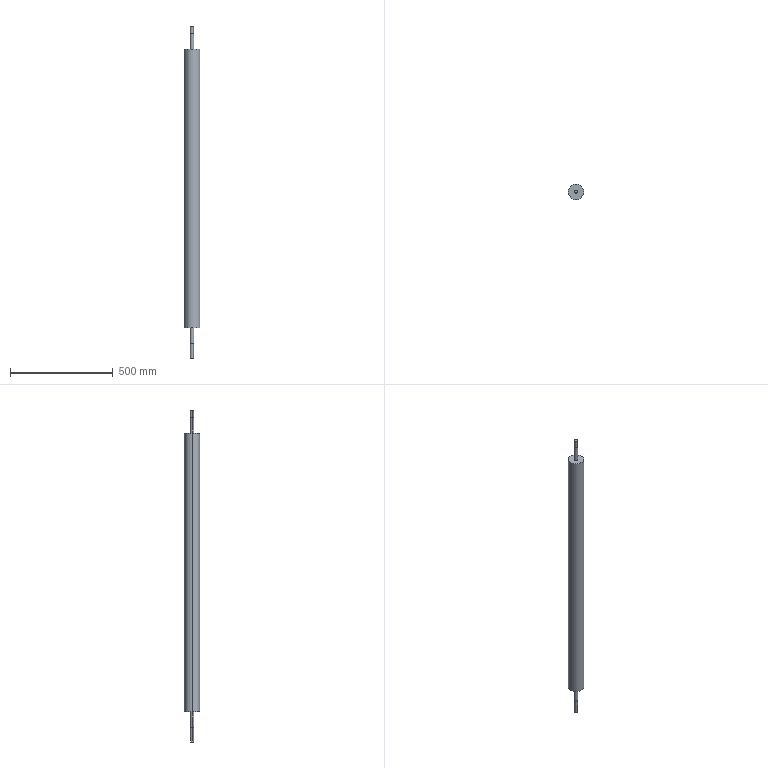Part | SolidWorks | features ICE 5, MirrorPattern 2, Extrusion 1 | 1 solid | 21 faces | box 76 x 76 x 1615 mm | volume 6202615 mm3 | cylinder 12 | plane 9 | commonest cylinder face diameters 15 x4 16.5 x4 5 x2 76 x2
STEP:
#1=CARTESIAN_POINT('',(2.5,4.5,-809.75));
#2=VERTEX_POINT('',#1);
#3=CARTESIAN_POINT('',(0.,4.5,-807.25));
#4=VERTEX_POINT('',#3);
#5=CARTESIAN_POINT('',(0.,4.5,-809.75));
#6=DIRECTION('',(0.,-1.,0.));
#7=DIRECTION('',(0.,0.,-1.));
#8=AXIS2_PLACEMENT_3D('',#5,#6,#7);
#9=CIRCLE('',#8,2.5);
#10=EDGE_CURVE('',#2,#4,#9,.T.);
#11=ORIENTED_EDGE('',*,*,#10,.T.);
#12=CARTESIAN_POINT('',(0.,7.5,-807.25));
#13=VERTEX_POINT('',#12);
#14=CARTESIAN_POINT('',(0.,4.5,-807.25));
#15=DIRECTION('',(0.,1.,0.));
#16=VECTOR('',#15,1000.);
#17=LINE('',#14,#16);
#18=EDGE_CURVE('',#4,#13,#17,.T.);
#19=ORIENTED_EDGE('',*,*,#18,.T.);
#20=CARTESIAN_POINT('',(2.5,7.071,-809.75));
#21=VERTEX_POINT('',#20);
#22=CARTESIAN_POINT('',(2.5,7.071,-809.75));
#23=CARTESIAN_POINT('',(2.5,7.071,-809.583));
#24=CARTESIAN_POINT('',(2.484,7.077,-809.42));
#25=CARTESIAN_POINT('',(2.419,7.099,-809.099));
#26=CARTESIAN_POINT('',(2.371,7.116,-808.939));
#27=CARTESIAN_POINT('',(2.245,7.157,-808.637));
#28=CARTESIAN_POINT('',(2.168,7.181,-808.494));
#29=CARTESIAN_POINT('',(1.986,7.233,-808.223));
#30=CARTESIAN_POINT('',(1.882,7.261,-808.096));
#31=CARTESIAN_POINT('',(1.538,7.344,-807.753));
#32=CARTESIAN_POINT('',(1.261,7.399,-807.567));
#33=CARTESIAN_POINT('',(0.81,7.458,-807.379));
#34=CARTESIAN_POINT('',(0.6511,7.473,-807.331));
#35=CARTESIAN_POINT('',(0.3276,7.495,-807.266));
#36=CARTESIAN_POINT('',(0.1645,7.5,-807.25));
#37=CARTESIAN_POINT('',(0.,7.5,-807.25));
#38=B_SPLINE_CURVE_WITH_KNOTS('',3,(#22,#23,#24,#25,#26,#27,#28,#29,#30,#31,#32,#33,#34,#35,#36,#37),.UNSPECIFIED.,.F.,.F.,(4,2,2,2,2,2,2,4),(0.,0.0004922,0.0009844,0.001477,0.001969,0.002953,0.003445,0.003937),.UNSPECIFIED.);
#39=EDGE_CURVE('',#21,#13,#38,.T.);
#40=ORIENTED_EDGE('',*,*,#39,.F.);
#41=CARTESIAN_POINT('',(2.5,4.5,-809.75));
#42=DIRECTION('',(0.,1.,0.));
#43=VECTOR('',#42,1000.);
#44=LINE('',#41,#43);
#45=EDGE_CURVE('',#2,#21,#44,.T.);
#46=ORIENTED_EDGE('',*,*,#45,.F.);
#47=EDGE_LOOP('',(#11,#19,#40,#46));
#48=FACE_OUTER_BOUND('',#47,.T.);
#49=CARTESIAN_POINT('',(0.,4.5,-809.75));
#50=DIRECTION('',(0.,1.,0.));
#51=DIRECTION('',(0.,0.,1.));
#52=AXIS2_PLACEMENT_3D('',#49,#50,#51);
#53=CYLINDRICAL_SURFACE('',#52,2.5);
#54=ADVANCED_FACE('',(#48),#53,.F.);
#55=CARTESIAN_POINT('',(-8.25,0.,-754.));
#56=VERTEX_POINT('',#55);
#57=CARTESIAN_POINT('',(8.25,0.,-754.));
#58=VERTEX_POINT('',#57);
#59=CARTESIAN_POINT('',(0.,0.,-754.));
#60=DIRECTION('',(0.,0.,-1.));
#61=DIRECTION('',(-1.,0.,0.));
#62=AXIS2_PLACEMENT_3D('',#59,#60,#61);
#63=CIRCLE('',#62,8.25);
#64=EDGE_CURVE('',#56,#58,#63,.T.);
#65=ORIENTED_EDGE('',*,*,#64,.F.);
#66=CARTESIAN_POINT('',(-8.25,0.,-678.));
#67=VERTEX_POINT('',#66);
#68=CARTESIAN_POINT('',(-8.25,0.,-754.));
#69=DIRECTION('',(0.,0.,1.));
#70=VECTOR('',#69,1000.);
#71=LINE('',#68,#70);
#72=EDGE_CURVE('',#56,#67,#71,.T.);
#73=ORIENTED_EDGE('',*,*,#72,.T.);
#74=CARTESIAN_POINT('',(8.25,0.,-678.));
#75=VERTEX_POINT('',#74);
#76=CARTESIAN_POINT('',(0.,0.,-678.));
#77=DIRECTION('',(0.,0.,-1.));
#78=DIRECTION('',(1.,0.,0.));
#79=AXIS2_PLACEMENT_3D('',#76,#77,#78);
#80=CIRCLE('',#79,8.25);
#81=EDGE_CURVE('',#67,#75,#80,.T.);
#82=ORIENTED_EDGE('',*,*,#81,.T.);
#83=CARTESIAN_POINT('',(8.25,0.,-754.));
#84=DIRECTION('',(0.,0.,1.));
#85=VECTOR('',#84,1000.);
#86=LINE('',#83,#85);
#87=EDGE_CURVE('',#58,#75,#86,.T.);
#88=ORIENTED_EDGE('',*,*,#87,.F.);
#89=EDGE_LOOP('',(#65,#73,#82,#88));
#90=FACE_OUTER_BOUND('',#89,.T.);
#91=CARTESIAN_POINT('',(0.,0.,-754.));
#92=DIRECTION('',(0.,0.,1.));
#93=DIRECTION('',(1.,0.,0.));
#94=AXIS2_PLACEMENT_3D('',#91,#92,#93);
#95=CYLINDRICAL_SURFACE('',#94,8.25);
#96=ADVANCED_FACE('',(#90),#95,.T.);
#97=CARTESIAN_POINT('',(8.25,0.,754.));
#98=VERTEX_POINT('',#97);
#99=CARTESIAN_POINT('',(-8.25,0.,754.));
#100=VERTEX_POINT('',#99);
#101=CARTESIAN_POINT('',(0.,0.,754.));
#102=DIRECTION('',(0.,0.,1.));
#103=DIRECTION('',(1.,0.,0.));
#104=AXIS2_PLACEMENT_3D('',#101,#102,#103);
#105=CIRCLE('',#104,8.25);
#106=EDGE_CURVE('',#98,#100,#105,.T.);
#107=ORIENTED_EDGE('',*,*,#106,.F.);
#108=CARTESIAN_POINT('',(8.25,0.,678.));
#109=VERTEX_POINT('',#108);
#110=CARTESIAN_POINT('',(8.25,0.,754.));
#111=DIRECTION('',(0.,0.,-1.));
#112=VECTOR('',#111,1000.);
#113=LINE('',#110,#112);
#114=EDGE_CURVE('',#98,#109,#113,.T.);
#115=ORIENTED_EDGE('',*,*,#114,.T.);
#116=CARTESIAN_POINT('',(-8.25,0.,678.));
#117=VERTEX_POINT('',#116);
#118=CARTESIAN_POINT('',(0.,0.,678.));
#119=DIRECTION('',(0.,0.,1.));
#120=DIRECTION('',(1.,0.,0.));
#121=AXIS2_PLACEMENT_3D('',#118,#119,#120);
#122=CIRCLE('',#121,8.25);
#123=EDGE_CURVE('',#109,#117,#122,.T.);
#124=ORIENTED_EDGE('',*,*,#123,.T.);
#125=CARTESIAN_POINT('',(-8.25,0.,754.));
#126=DIRECTION('',(0.,0.,-1.));
#127=VECTOR('',#126,1000.);
#128=LINE('',#125,#127);
#129=EDGE_CURVE('',#100,#117,#128,.T.);
#130=ORIENTED_EDGE('',*,*,#129,.F.);
#131=EDGE_LOOP('',(#107,#115,#124,#130));
#132=FACE_OUTER_BOUND('',#131,.T.);
#133=CARTESIAN_POINT('',(0.,0.,754.));
#134=DIRECTION('',(0.,0.,-1.));
#135=DIRECTION('',(-1.,0.,0.));
#136=AXIS2_PLACEMENT_3D('',#133,#134,#135);
#137=CYLINDRICAL_SURFACE('',#136,8.25);
#138=ADVANCED_FACE('',(#132),#137,.T.);
#139=CARTESIAN_POINT('',(38.,0.,678.));
#140=VERTEX_POINT('',#139);
#141=CARTESIAN_POINT('',(-38.,0.,678.));
#142=VERTEX_POINT('',#141);
#143=CARTESIAN_POINT('',(0.,0.,678.));
#144=DIRECTION('',(0.,0.,1.));
#145=DIRECTION('',(1.,0.,0.));
#146=AXIS2_PLACEMENT_3D('',#143,#144,#145);
#147=CIRCLE('',#146,38.);
#148=EDGE_CURVE('',#140,#142,#147,.T.);
#149=ORIENTED_EDGE('',*,*,#148,.F.);
#150=CARTESIAN_POINT('',(38.,0.,-678.));
#151=VERTEX_POINT('',#150);
#152=CARTESIAN_POINT('',(38.,0.,678.));
#153=DIRECTION('',(0.,0.,-1.));
#154=VECTOR('',#153,1000.);
#155=LINE('',#152,#154);
#156=EDGE_CURVE('',#140,#151,#155,.T.);
#157=ORIENTED_EDGE('',*,*,#156,.T.);
#158=CARTESIAN_POINT('',(-38.,0.,-678.));
#159=VERTEX_POINT('',#158);
#160=CARTESIAN_POINT('',(0.,0.,-678.));
#161=DIRECTION('',(0.,0.,1.));
#162=DIRECTION('',(1.,0.,0.));
#163=AXIS2_PLACEMENT_3D('',#160,#161,#162);
#164=CIRCLE('',#163,38.);
#165=EDGE_CURVE('',#151,#159,#164,.T.);
#166=ORIENTED_EDGE('',*,*,#165,.T.);
#167=CARTESIAN_POINT('',(-38.,0.,678.));
#168=DIRECTION('',(0.,0.,-1.));
#169=VECTOR('',#168,1000.);
#170=LINE('',#167,#169);
#171=EDGE_CURVE('',#142,#159,#170,.T.);
#172=ORIENTED_EDGE('',*,*,#171,.F.);
#173=EDGE_LOOP('',(#149,#157,#166,#172));
#174=FACE_OUTER_BOUND('',#173,.T.);
#175=CARTESIAN_POINT('',(0.,0.,678.));
#176=DIRECTION('',(0.,0.,-1.));
#177=DIRECTION('',(-1.,0.,0.));
#178=AXIS2_PLACEMENT_3D('',#175,#176,#177);
#179=CYLINDRICAL_SURFACE('',#178,38.);
#180=ADVANCED_FACE('',(#174),#179,.T.);
#181=CARTESIAN_POINT('',(-2.5,7.071,-824.75));
#182=VERTEX_POINT('',#181);
#183=CARTESIAN_POINT('',(-7.5,0.,-824.75));
#184=VERTEX_POINT('',#183);
#185=CARTESIAN_POINT('',(0.,0.,-824.75));
#186=DIRECTION('',(0.,0.,1.));
#187=DIRECTION('',(1.,0.,0.));
#188=AXIS2_PLACEMENT_3D('',#185,#186,#187);
#189=CIRCLE('',#188,7.5);
#190=EDGE_CURVE('',#182,#184,#189,.T.);
#191=ORIENTED_EDGE('',*,*,#190,.T.);
#192=CARTESIAN_POINT('',(-7.5,0.,-754.));
#193=VERTEX_POINT('',#192);
#194=CARTESIAN_POINT('',(-7.5,0.,-824.75));
#195=DIRECTION('',(0.,0.,1.));
#196=VECTOR('',#195,1000.);
#197=LINE('',#194,#196);
#198=EDGE_CURVE('',#184,#193,#197,.T.);
#199=ORIENTED_EDGE('',*,*,#198,.T.);
#200=CARTESIAN_POINT('',(7.5,0.,-754.));
#201=VERTEX_POINT('',#200);
#202=CARTESIAN_POINT('',(0.,0.,-754.));
#203=DIRECTION('',(0.,0.,1.));
#204=DIRECTION('',(-1.,0.,0.));
#205=AXIS2_PLACEMENT_3D('',#202,#203,#204);
#206=CIRCLE('',#205,7.5);
#207=EDGE_CURVE('',#201,#193,#206,.T.);
#208=ORIENTED_EDGE('',*,*,#207,.F.);
#209=CARTESIAN_POINT('',(7.5,0.,-824.75));
#210=VERTEX_POINT('',#209);
#211=CARTESIAN_POINT('',(7.5,0.,-824.75));
#212=DIRECTION('',(0.,0.,1.));
#213=VECTOR('',#212,1000.);
#214=LINE('',#211,#213);
#215=EDGE_CURVE('',#210,#201,#214,.T.);
#216=ORIENTED_EDGE('',*,*,#215,.F.);
#217=CARTESIAN_POINT('',(2.5,7.071,-824.75));
#218=VERTEX_POINT('',#217);
#219=CARTESIAN_POINT('',(0.,0.,-824.75));
#220=DIRECTION('',(0.,0.,1.));
#221=DIRECTION('',(1.,0.,0.));
#222=AXIS2_PLACEMENT_3D('',#219,#220,#221);
#223=CIRCLE('',#222,7.5);
#224=EDGE_CURVE('',#210,#218,#223,.T.);
#225=ORIENTED_EDGE('',*,*,#224,.T.);
#226=CARTESIAN_POINT('',(2.5,7.071,-824.75));
#227=DIRECTION('',(0.,0.,1.));
#228=VECTOR('',#227,1000.);
#229=LINE('',#226,#228);
#230=EDGE_CURVE('',#218,#21,#229,.T.);
#231=ORIENTED_EDGE('',*,*,#230,.T.);
#232=ORIENTED_EDGE('',*,*,#39,.T.);
#233=CARTESIAN_POINT('',(-2.5,7.071,-809.75));
#234=VERTEX_POINT('',#233);
#235=CARTESIAN_POINT('',(0.,7.5,-807.25));
#236=CARTESIAN_POINT('',(-0.1643,7.5,-807.25));
#237=CARTESIAN_POINT('',(-0.3311,7.494,-807.267));
#238=CARTESIAN_POINT('',(-0.6524,7.473,-807.331));
#239=CARTESIAN_POINT('',(-0.8088,7.458,-807.379));
#240=CARTESIAN_POINT('',(-1.113,7.419,-807.505));
#241=CARTESIAN_POINT('',(-1.257,7.395,-807.583));
#242=CARTESIAN_POINT('',(-1.526,7.344,-807.763));
#243=CARTESIAN_POINT('',(-1.653,7.316,-807.868));
#244=CARTESIAN_POINT('',(-1.883,7.261,-808.098));
#245=CARTESIAN_POINT('',(-1.986,7.233,-808.223));
#246=CARTESIAN_POINT('',(-2.167,7.181,-808.492));
#247=CARTESIAN_POINT('',(-2.245,7.156,-808.638));
#248=CARTESIAN_POINT('',(-2.37,7.116,-808.939));
#249=CARTESIAN_POINT('',(-2.418,7.1,-809.094));
#250=CARTESIAN_POINT('',(-2.483,7.077,-809.418));
#251=CARTESIAN_POINT('',(-2.5,7.071,-809.584));
#252=CARTESIAN_POINT('',(-2.5,7.071,-809.75));
#253=B_SPLINE_CURVE_WITH_KNOTS('',3,(#235,#236,#237,#238,#239,#240,#241,#242,#243,#244,#245,#246,#247,#248,#249,#250,#251,#252),.UNSPECIFIED.,.F.,.F.,(4,2,2,2,2,2,2,2,4),(0.003937,0.004429,0.004921,0.005412,0.005904,0.006395,0.006887,0.007378,0.00787),.UNSPECIFIED.);
#254=EDGE_CURVE('',#13,#234,#253,.T.);
#255=ORIENTED_EDGE('',*,*,#254,.T.);
#256=CARTESIAN_POINT('',(-2.5,7.071,-824.75));
#257=DIRECTION('',(0.,0.,-1.));
#258=VECTOR('',#257,1000.);
#259=LINE('',#256,#258);
#260=EDGE_CURVE('',#234,#182,#259,.T.);
#261=ORIENTED_EDGE('',*,*,#260,.T.);
#262=EDGE_LOOP('',(#191,#199,#208,#216,#225,#231,#232,#255,#261));
#263=FACE_OUTER_BOUND('',#262,.T.);
#264=CARTESIAN_POINT('',(0.,0.,-824.75));
#265=DIRECTION('',(0.,0.,1.));
#266=DIRECTION('',(1.,0.,0.));
#267=AXIS2_PLACEMENT_3D('',#264,#265,#266);
#268=CYLINDRICAL_SURFACE('',#267,7.5);
#269=ADVANCED_FACE('',(#263),#268,.T.);
#270=CARTESIAN_POINT('',(7.5,0.,790.3));
#271=VERTEX_POINT('',#270);
#272=CARTESIAN_POINT('',(-7.5,0.,790.3));
#273=VERTEX_POINT('',#272);
#274=CARTESIAN_POINT('',(0.,0.,790.3));
#275=DIRECTION('',(0.,0.,1.));
#276=DIRECTION('',(1.,0.,0.));
#277=AXIS2_PLACEMENT_3D('',#274,#275,#276);
#278=CIRCLE('',#277,7.5);
#279=EDGE_CURVE('',#271,#273,#278,.T.);
#280=ORIENTED_EDGE('',*,*,#279,.F.);
#281=CARTESIAN_POINT('',(7.5,0.,754.));
#282=VERTEX_POINT('',#281);
#283=CARTESIAN_POINT('',(7.5,0.,824.75));
#284=DIRECTION('',(0.,0.,-1.));
#285=VECTOR('',#284,1000.);
#286=LINE('',#283,#285);
#287=EDGE_CURVE('',#271,#282,#286,.T.);
#288=ORIENTED_EDGE('',*,*,#287,.T.);
#289=CARTESIAN_POINT('',(-7.5,0.,754.));
#290=VERTEX_POINT('',#289);
#291=CARTESIAN_POINT('',(0.,0.,754.));
#292=DIRECTION('',(0.,0.,1.));
#293=DIRECTION('',(1.,0.,0.));
#294=AXIS2_PLACEMENT_3D('',#291,#292,#293);
#295=CIRCLE('',#294,7.5);
#296=EDGE_CURVE('',#282,#290,#295,.T.);
#297=ORIENTED_EDGE('',*,*,#296,.T.);
#298=CARTESIAN_POINT('',(-7.5,0.,824.75));
#299=DIRECTION('',(0.,0.,-1.));
#300=VECTOR('',#299,1000.);
#301=LINE('',#298,#300);
#302=EDGE_CURVE('',#273,#290,#301,.T.);
#303=ORIENTED_EDGE('',*,*,#302,.F.);
#304=EDGE_LOOP('',(#280,#288,#297,#303));
#305=FACE_OUTER_BOUND('',#304,.T.);
#306=CARTESIAN_POINT('',(0.,0.,824.75));
#307=DIRECTION('',(0.,0.,-1.));
#308=DIRECTION('',(-1.,0.,0.));
#309=AXIS2_PLACEMENT_3D('',#306,#307,#308);
#310=CYLINDRICAL_SURFACE('',#309,7.5);
#311=ADVANCED_FACE('',(#305),#310,.T.);
#312=ORIENTED_EDGE('',*,*,#287,.F.);
#313=CARTESIAN_POINT('',(0.,0.,790.3));
#314=DIRECTION('',(0.,0.,1.));
#315=DIRECTION('',(1.,0.,0.));
#316=AXIS2_PLACEMENT_3D('',#313,#314,#315);
#317=CIRCLE('',#316,7.5);
#318=EDGE_CURVE('',#273,#271,#317,.T.);
#319=ORIENTED_EDGE('',*,*,#318,.F.);
#320=ORIENTED_EDGE('',*,*,#302,.T.);
#321=CARTESIAN_POINT('',(0.,0.,754.));
#322=DIRECTION('',(0.,0.,1.));
#323=DIRECTION('',(1.,0.,0.));
#324=AXIS2_PLACEMENT_3D('',#321,#322,#323);
#325=CIRCLE('',#324,7.5);
#326=EDGE_CURVE('',#290,#282,#325,.T.);
#327=ORIENTED_EDGE('',*,*,#326,.T.);
#328=EDGE_LOOP('',(#312,#319,#320,#327));
#329=FACE_OUTER_BOUND('',#328,.T.);
#330=CARTESIAN_POINT('',(0.,0.,824.75));
#331=DIRECTION('',(0.,0.,-1.));
#332=DIRECTION('',(-1.,0.,0.));
#333=AXIS2_PLACEMENT_3D('',#330,#331,#332);
#334=CYLINDRICAL_SURFACE('',#333,7.5);
#335=ADVANCED_FACE('',(#329),#334,.T.);
#336=CARTESIAN_POINT('',(-2.5,4.5,-824.75));
#337=VERTEX_POINT('',#336);
#338=CARTESIAN_POINT('',(2.5,4.5,-824.75));
#339=VERTEX_POINT('',#338);
#340=CARTESIAN_POINT('',(0.,4.5,-824.75));
#341=DIRECTION('',(1.,0.,0.));
#342=VECTOR('',#341,1000.);
#343=LINE('',#340,#342);
#344=EDGE_CURVE('',#337,#339,#343,.T.);
#345=ORIENTED_EDGE('',*,*,#344,.T.);
#346=CARTESIAN_POINT('',(2.5,4.5,-824.75));
#347=DIRECTION('',(0.,1.,0.));
#348=VECTOR('',#347,1000.);
#349=LINE('',#346,#348);
#350=EDGE_CURVE('',#339,#218,#349,.T.);
#351=ORIENTED_EDGE('',*,*,#350,.T.);
#352=ORIENTED_EDGE('',*,*,#224,.F.);
#353=CARTESIAN_POINT('',(0.,0.,-824.75));
#354=DIRECTION('',(0.,0.,1.));
#355=DIRECTION('',(1.,0.,0.));
#356=AXIS2_PLACEMENT_3D('',#353,#354,#355);
#357=CIRCLE('',#356,7.5);
#358=EDGE_CURVE('',#184,#210,#357,.T.);
#359=ORIENTED_EDGE('',*,*,#358,.F.);
#360=ORIENTED_EDGE('',*,*,#190,.F.);
#361=CARTESIAN_POINT('',(-2.5,4.5,-824.75));
#362=DIRECTION('',(0.,1.,0.));
#363=VECTOR('',#362,1000.);
#364=LINE('',#361,#363);
#365=EDGE_CURVE('',#337,#182,#364,.T.);
#366=ORIENTED_EDGE('',*,*,#365,.F.);
#367=EDGE_LOOP('',(#345,#351,#352,#359,#360,#366));
#368=FACE_OUTER_BOUND('',#367,.T.);
#369=CARTESIAN_POINT('',(0.,0.,-824.75));
#370=DIRECTION('',(0.,0.,-1.));
#371=DIRECTION('',(1.,0.,0.));
#372=AXIS2_PLACEMENT_3D('',#369,#370,#371);
#373=PLANE('',#372);
#374=ADVANCED_FACE('',(#368),#373,.T.);
#375=ORIENTED_EDGE('',*,*,#198,.F.);
#376=ORIENTED_EDGE('',*,*,#358,.T.);
#377=ORIENTED_EDGE('',*,*,#215,.T.);
#378=CARTESIAN_POINT('',(0.,0.,-754.));
#379=DIRECTION('',(0.,0.,1.));
#380=DIRECTION('',(-1.,0.,0.));
#381=AXIS2_PLACEMENT_3D('',#378,#379,#380);
#382=CIRCLE('',#381,7.5);
#383=EDGE_CURVE('',#193,#201,#382,.T.);
#384=ORIENTED_EDGE('',*,*,#383,.F.);
#385=EDGE_LOOP('',(#375,#376,#377,#384));
#386=FACE_OUTER_BOUND('',#385,.T.);
#387=CARTESIAN_POINT('',(0.,0.,-824.75));
#388=DIRECTION('',(0.,0.,1.));
#389=DIRECTION('',(1.,0.,0.));
#390=AXIS2_PLACEMENT_3D('',#387,#388,#389);
#391=CYLINDRICAL_SURFACE('',#390,7.5);
#392=ADVANCED_FACE('',(#386),#391,.T.);
#393=ORIENTED_EDGE('',*,*,#156,.F.);
#394=CARTESIAN_POINT('',(0.,0.,678.));
#395=DIRECTION('',(0.,0.,1.));
#396=DIRECTION('',(1.,0.,0.));
#397=AXIS2_PLACEMENT_3D('',#394,#395,#396);
#398=CIRCLE('',#397,38.);
#399=EDGE_CURVE('',#142,#140,#398,.T.);
#400=ORIENTED_EDGE('',*,*,#399,.F.);
#401=ORIENTED_EDGE('',*,*,#171,.T.);
#402=CARTESIAN_POINT('',(0.,0.,-678.));
#403=DIRECTION('',(0.,0.,1.));
#404=DIRECTION('',(1.,0.,0.));
#405=AXIS2_PLACEMENT_3D('',#402,#403,#404);
#406=CIRCLE('',#405,38.);
#407=EDGE_CURVE('',#159,#151,#406,.T.);
#408=ORIENTED_EDGE('',*,*,#407,.T.);
#409=EDGE_LOOP('',(#393,#400,#401,#408));
#410=FACE_OUTER_BOUND('',#409,.T.);
#411=CARTESIAN_POINT('',(0.,0.,678.));
#412=DIRECTION('',(0.,0.,-1.));
#413=DIRECTION('',(-1.,0.,0.));
#414=AXIS2_PLACEMENT_3D('',#411,#412,#413);
#415=CYLINDRICAL_SURFACE('',#414,38.);
#416=ADVANCED_FACE('',(#410),#415,.T.);
#417=CARTESIAN_POINT('',(0.,0.,678.));
#418=DIRECTION('',(0.,0.,1.));
#419=DIRECTION('',(1.,0.,0.));
#420=AXIS2_PLACEMENT_3D('',#417,#418,#419);
#421=CIRCLE('',#420,8.25);
#422=EDGE_CURVE('',#117,#109,#421,.T.);
#423=ORIENTED_EDGE('',*,*,#422,.F.);
#424=ORIENTED_EDGE('',*,*,#123,.F.);
#425=EDGE_LOOP('',(#423,#424));
#426=FACE_BOUND('',#425,.T.);
#427=ORIENTED_EDGE('',*,*,#399,.T.);
#428=ORIENTED_EDGE('',*,*,#148,.T.);
#429=EDGE_LOOP('',(#427,#428));
#430=FACE_OUTER_BOUND('',#429,.T.);
#431=CARTESIAN_POINT('',(0.,0.,678.));
#432=DIRECTION('',(0.,0.,1.));
#433=DIRECTION('',(1.,0.,0.));
#434=AXIS2_PLACEMENT_3D('',#431,#432,#433);
#435=PLANE('',#434);
#436=ADVANCED_FACE('',(#426,#430),#435,.T.);
#437=CARTESIAN_POINT('',(0.,0.,-678.));
#438=DIRECTION('',(0.,0.,-1.));
#439=DIRECTION('',(1.,0.,0.));
#440=AXIS2_PLACEMENT_3D('',#437,#438,#439);
#441=CIRCLE('',#440,8.25);
#442=EDGE_CURVE('',#75,#67,#441,.T.);
#443=ORIENTED_EDGE('',*,*,#442,.F.);
#444=ORIENTED_EDGE('',*,*,#81,.F.);
#445=EDGE_LOOP('',(#443,#444));
#446=FACE_BOUND('',#445,.T.);
#447=ORIENTED_EDGE('',*,*,#407,.F.);
#448=ORIENTED_EDGE('',*,*,#165,.F.);
#449=EDGE_LOOP('',(#447,#448));
#450=FACE_OUTER_BOUND('',#449,.T.);
#451=CARTESIAN_POINT('',(0.,0.,-678.));
#452=DIRECTION('',(0.,0.,1.));
#453=DIRECTION('',(1.,0.,0.));
#454=AXIS2_PLACEMENT_3D('',#451,#452,#453);
#455=PLANE('',#454);
#456=ADVANCED_FACE('',(#446,#450),#455,.F.);
#457=ORIENTED_EDGE('',*,*,#114,.F.);
#458=CARTESIAN_POINT('',(0.,0.,754.));
#459=DIRECTION('',(0.,0.,1.));
#460=DIRECTION('',(1.,0.,0.));
#461=AXIS2_PLACEMENT_3D('',#458,#459,#460);
#462=CIRCLE('',#461,8.25);
#463=EDGE_CURVE('',#100,#98,#462,.T.);
#464=ORIENTED_EDGE('',*,*,#463,.F.);
#465=ORIENTED_EDGE('',*,*,#129,.T.);
#466=ORIENTED_EDGE('',*,*,#422,.T.);
#467=EDGE_LOOP('',(#457,#464,#465,#466));
#468=FACE_OUTER_BOUND('',#467,.T.);
#469=CARTESIAN_POINT('',(0.,0.,754.));
#470=DIRECTION('',(0.,0.,-1.));
#471=DIRECTION('',(-1.,0.,0.));
#472=AXIS2_PLACEMENT_3D('',#469,#470,#471);
#473=CYLINDRICAL_SURFACE('',#472,8.25);
#474=ADVANCED_FACE('',(#468),#473,.T.);
#475=ORIENTED_EDGE('',*,*,#326,.F.);
#476=ORIENTED_EDGE('',*,*,#296,.F.);
#477=EDGE_LOOP('',(#475,#476));
#478=FACE_BOUND('',#477,.T.);
#479=ORIENTED_EDGE('',*,*,#463,.T.);
#480=ORIENTED_EDGE('',*,*,#106,.T.);
#481=EDGE_LOOP('',(#479,#480));
#482=FACE_OUTER_BOUND('',#481,.T.);
#483=CARTESIAN_POINT('',(0.,0.,754.));
#484=DIRECTION('',(0.,0.,1.));
#485=DIRECTION('',(1.,0.,0.));
#486=AXIS2_PLACEMENT_3D('',#483,#484,#485);
#487=PLANE('',#486);
#488=ADVANCED_FACE('',(#478,#482),#487,.T.);
#489=ORIENTED_EDGE('',*,*,#72,.F.);
#490=CARTESIAN_POINT('',(0.,0.,-754.));
#491=DIRECTION('',(0.,0.,-1.));
#492=DIRECTION('',(-1.,0.,0.));
#493=AXIS2_PLACEMENT_3D('',#490,#491,#492);
#494=CIRCLE('',#493,8.25);
#495=EDGE_CURVE('',#58,#56,#494,.T.);
#496=ORIENTED_EDGE('',*,*,#495,.F.);
#497=ORIENTED_EDGE('',*,*,#87,.T.);
#498=ORIENTED_EDGE('',*,*,#442,.T.);
#499=EDGE_LOOP('',(#489,#496,#497,#498));
#500=FACE_OUTER_BOUND('',#499,.T.);
#501=CARTESIAN_POINT('',(0.,0.,-754.));
#502=DIRECTION('',(0.,0.,1.));
#503=DIRECTION('',(1.,0.,0.));
#504=AXIS2_PLACEMENT_3D('',#501,#502,#503);
#505=CYLINDRICAL_SURFACE('',#504,8.25);
#506=ADVANCED_FACE('',(#500),#505,.T.);
#507=ORIENTED_EDGE('',*,*,#207,.T.);
#508=ORIENTED_EDGE('',*,*,#383,.T.);
#509=EDGE_LOOP('',(#507,#508));
#510=FACE_BOUND('',#509,.T.);
#511=ORIENTED_EDGE('',*,*,#495,.T.);
#512=ORIENTED_EDGE('',*,*,#64,.T.);
#513=EDGE_LOOP('',(#511,#512));
#514=FACE_OUTER_BOUND('',#513,.T.);
#515=CARTESIAN_POINT('',(0.,0.,-754.));
#516=DIRECTION('',(0.,0.,-1.));
#517=DIRECTION('',(-1.,0.,0.));
#518=AXIS2_PLACEMENT_3D('',#515,#516,#517);
#519=PLANE('',#518);
#520=ADVANCED_FACE('',(#510,#514),#519,.T.);
#521=ORIENTED_EDGE('',*,*,#350,.F.);
#522=CARTESIAN_POINT('',(2.5,4.5,-824.75));
#523=DIRECTION('',(0.,0.,1.));
#524=VECTOR('',#523,1000.);
#525=LINE('',#522,#524);
#526=EDGE_CURVE('',#339,#2,#525,.T.);
#527=ORIENTED_EDGE('',*,*,#526,.T.);
#528=ORIENTED_EDGE('',*,*,#45,.T.);
#529=ORIENTED_EDGE('',*,*,#230,.F.);
#530=EDGE_LOOP('',(#521,#527,#528,#529));
#531=FACE_OUTER_BOUND('',#530,.T.);
#532=CARTESIAN_POINT('',(2.5,4.5,-824.75));
#533=DIRECTION('',(-1.,0.,0.));
#534=DIRECTION('',(0.,0.,1.));
#535=AXIS2_PLACEMENT_3D('',#532,#533,#534);
#536=PLANE('',#535);
#537=ADVANCED_FACE('',(#531),#536,.T.);
#538=ORIENTED_EDGE('',*,*,#18,.F.);
#539=CARTESIAN_POINT('',(-2.5,4.5,-809.75));
#540=VERTEX_POINT('',#539);
#541=CARTESIAN_POINT('',(0.,4.5,-809.75));
#542=DIRECTION('',(0.,-1.,0.));
#543=DIRECTION('',(0.,0.,-1.));
#544=AXIS2_PLACEMENT_3D('',#541,#542,#543);
#545=CIRCLE('',#544,2.5);
#546=EDGE_CURVE('',#4,#540,#545,.T.);
#547=ORIENTED_EDGE('',*,*,#546,.T.);
#548=CARTESIAN_POINT('',(-2.5,4.5,-809.75));
#549=DIRECTION('',(0.,1.,0.));
#550=VECTOR('',#549,1000.);
#551=LINE('',#548,#550);
#552=EDGE_CURVE('',#540,#234,#551,.T.);
#553=ORIENTED_EDGE('',*,*,#552,.T.);
#554=ORIENTED_EDGE('',*,*,#254,.F.);
#555=EDGE_LOOP('',(#538,#547,#553,#554));
#556=FACE_OUTER_BOUND('',#555,.T.);
#557=CARTESIAN_POINT('',(0.,4.5,-809.75));
#558=DIRECTION('',(0.,1.,0.));
#559=DIRECTION('',(0.,0.,1.));
#560=AXIS2_PLACEMENT_3D('',#557,#558,#559);
#561=CYLINDRICAL_SURFACE('',#560,2.5);
#562=ADVANCED_FACE('',(#556),#561,.F.);
#563=ORIENTED_EDGE('',*,*,#552,.F.);
#564=CARTESIAN_POINT('',(-2.5,4.5,-824.75));
#565=DIRECTION('',(0.,0.,-1.));
#566=VECTOR('',#565,1000.);
#567=LINE('',#564,#566);
#568=EDGE_CURVE('',#540,#337,#567,.T.);
#569=ORIENTED_EDGE('',*,*,#568,.T.);
#570=ORIENTED_EDGE('',*,*,#365,.T.);
#571=ORIENTED_EDGE('',*,*,#260,.F.);
#572=EDGE_LOOP('',(#563,#569,#570,#571));
#573=FACE_OUTER_BOUND('',#572,.T.);
#574=CARTESIAN_POINT('',(-2.5,4.5,-824.75));
#575=DIRECTION('',(1.,0.,0.));
#576=DIRECTION('',(0.,0.,-1.));
#577=AXIS2_PLACEMENT_3D('',#574,#575,#576);
#578=PLANE('',#577);
#579=ADVANCED_FACE('',(#573),#578,.T.);
#580=ORIENTED_EDGE('',*,*,#568,.F.);
#581=ORIENTED_EDGE('',*,*,#546,.F.);
#582=ORIENTED_EDGE('',*,*,#10,.F.);
#583=ORIENTED_EDGE('',*,*,#526,.F.);
#584=ORIENTED_EDGE('',*,*,#344,.F.);
#585=EDGE_LOOP('',(#580,#581,#582,#583,#584));
#586=FACE_OUTER_BOUND('',#585,.T.);
#587=CARTESIAN_POINT('',(0.,4.5,-824.75));
#588=DIRECTION('',(0.,1.,0.));
#589=DIRECTION('',(0.,0.,-1.));
#590=AXIS2_PLACEMENT_3D('',#587,#588,#589);
#591=PLANE('',#590);
#592=ADVANCED_FACE('',(#586),#591,.T.);
#593=ORIENTED_EDGE('',*,*,#318,.T.);
#594=ORIENTED_EDGE('',*,*,#279,.T.);
#595=EDGE_LOOP('',(#593,#594));
#596=FACE_OUTER_BOUND('',#595,.T.);
#597=CARTESIAN_POINT('',(0.,0.,790.3));
#598=DIRECTION('',(0.,0.,1.));
#599=DIRECTION('',(1.,0.,0.));
#600=AXIS2_PLACEMENT_3D('',#597,#598,#599);
#601=PLANE('',#600);
#602=ADVANCED_FACE('',(#596),#601,.T.);
#603=CLOSED_SHELL('',(#54,#96,#138,#180,#269,#311,#335,#374,#392,#416,#436,#456,#474,#488,#506,#520,#537,#562,#579,#592,#602));
#604=MANIFOLD_SOLID_BREP('',#603);
#605=CARTESIAN_POINT('',(0.,0.,0.));
#606=DIRECTION('',(0.,0.,1.));
#607=DIRECTION('',(1.,0.,0.));
#608=AXIS2_PLACEMENT_3D('',#605,#606,#607);
#609=(LENGTH_UNIT()NAMED_UNIT(*)SI_UNIT(.MILLI.,.METRE.));
#610=UNCERTAINTY_MEASURE_WITH_UNIT(LENGTH_MEASURE(0.00001),#609,'','');
#611=(NAMED_UNIT(*)PLANE_ANGLE_UNIT()SI_UNIT($,.RADIAN.));
#612=(NAMED_UNIT(*)SI_UNIT($,.STERADIAN.)SOLID_ANGLE_UNIT());
#613=(GEOMETRIC_REPRESENTATION_CONTEXT(3)GLOBAL_UNCERTAINTY_ASSIGNED_CONTEXT((#610))GLOBAL_UNIT_ASSIGNED_CONTEXT((#609,#611,#612))REPRESENTATION_CONTEXT('',''));
#614=ADVANCED_BREP_SHAPE_REPRESENTATION('',(#604,#608),#613);